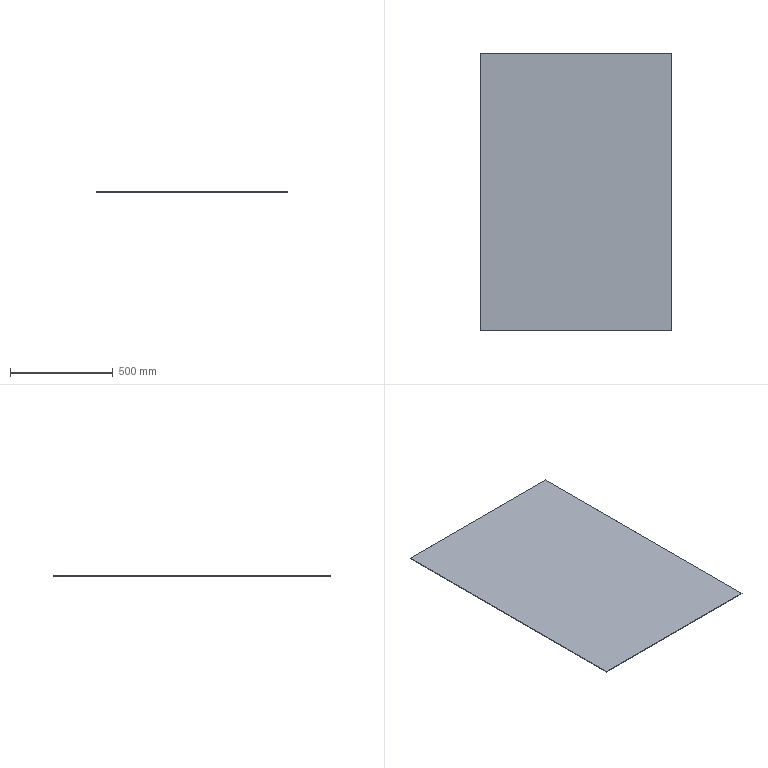Part | SolidWorks | features Extrusion 1 | 1 solid | 6 faces | box 935 x 1355 x 3 mm | volume 3800775 mm3 | plane 6
STEP:
#1=CARTESIAN_POINT('',(467.5,-677.5,0.));
#2=VERTEX_POINT('',#1);
#3=CARTESIAN_POINT('',(467.5,677.5,0.));
#4=VERTEX_POINT('',#3);
#5=CARTESIAN_POINT('',(467.5,677.5,0.));
#6=DIRECTION('',(0.,1.,0.));
#7=VECTOR('',#6,1000.);
#8=LINE('',#5,#7);
#9=EDGE_CURVE('',#2,#4,#8,.T.);
#10=ORIENTED_EDGE('',*,*,#9,.T.);
#11=CARTESIAN_POINT('',(467.5,677.5,3.));
#12=VERTEX_POINT('',#11);
#13=CARTESIAN_POINT('',(467.5,677.5,3.));
#14=DIRECTION('',(0.,0.,-1.));
#15=VECTOR('',#14,1000.);
#16=LINE('',#13,#15);
#17=EDGE_CURVE('',#12,#4,#16,.T.);
#18=ORIENTED_EDGE('',*,*,#17,.F.);
#19=CARTESIAN_POINT('',(467.5,-677.5,3.));
#20=VERTEX_POINT('',#19);
#21=CARTESIAN_POINT('',(467.5,677.5,3.));
#22=DIRECTION('',(0.,1.,0.));
#23=VECTOR('',#22,1000.);
#24=LINE('',#21,#23);
#25=EDGE_CURVE('',#20,#12,#24,.T.);
#26=ORIENTED_EDGE('',*,*,#25,.F.);
#27=CARTESIAN_POINT('',(467.5,-677.5,3.));
#28=DIRECTION('',(0.,0.,-1.));
#29=VECTOR('',#28,1000.);
#30=LINE('',#27,#29);
#31=EDGE_CURVE('',#20,#2,#30,.T.);
#32=ORIENTED_EDGE('',*,*,#31,.T.);
#33=EDGE_LOOP('',(#10,#18,#26,#32));
#34=FACE_OUTER_BOUND('',#33,.T.);
#35=CARTESIAN_POINT('',(467.5,677.5,3.));
#36=DIRECTION('',(-1.,0.,0.));
#37=DIRECTION('',(0.,-1.,0.));
#38=AXIS2_PLACEMENT_3D('',#35,#36,#37);
#39=PLANE('',#38);
#40=ADVANCED_FACE('',(#34),#39,.F.);
#41=CARTESIAN_POINT('',(-467.5,677.5,0.));
#42=VERTEX_POINT('',#41);
#43=CARTESIAN_POINT('',(-467.5,677.5,0.));
#44=DIRECTION('',(-1.,0.,0.));
#45=VECTOR('',#44,1000.);
#46=LINE('',#43,#45);
#47=EDGE_CURVE('',#4,#42,#46,.T.);
#48=ORIENTED_EDGE('',*,*,#47,.T.);
#49=CARTESIAN_POINT('',(-467.5,677.5,3.));
#50=VERTEX_POINT('',#49);
#51=CARTESIAN_POINT('',(-467.5,677.5,3.));
#52=DIRECTION('',(0.,0.,-1.));
#53=VECTOR('',#52,1000.);
#54=LINE('',#51,#53);
#55=EDGE_CURVE('',#50,#42,#54,.T.);
#56=ORIENTED_EDGE('',*,*,#55,.F.);
#57=CARTESIAN_POINT('',(-467.5,677.5,3.));
#58=DIRECTION('',(-1.,0.,0.));
#59=VECTOR('',#58,1000.);
#60=LINE('',#57,#59);
#61=EDGE_CURVE('',#12,#50,#60,.T.);
#62=ORIENTED_EDGE('',*,*,#61,.F.);
#63=ORIENTED_EDGE('',*,*,#17,.T.);
#64=EDGE_LOOP('',(#48,#56,#62,#63));
#65=FACE_OUTER_BOUND('',#64,.T.);
#66=CARTESIAN_POINT('',(-467.5,677.5,3.));
#67=DIRECTION('',(0.,-1.,0.));
#68=DIRECTION('',(0.,0.,-1.));
#69=AXIS2_PLACEMENT_3D('',#66,#67,#68);
#70=PLANE('',#69);
#71=ADVANCED_FACE('',(#65),#70,.F.);
#72=CARTESIAN_POINT('',(-467.5,-677.5,0.));
#73=VERTEX_POINT('',#72);
#74=CARTESIAN_POINT('',(-467.5,677.5,0.));
#75=DIRECTION('',(0.,-1.,0.));
#76=VECTOR('',#75,1000.);
#77=LINE('',#74,#76);
#78=EDGE_CURVE('',#42,#73,#77,.T.);
#79=ORIENTED_EDGE('',*,*,#78,.T.);
#80=CARTESIAN_POINT('',(-467.5,-677.5,3.));
#81=VERTEX_POINT('',#80);
#82=CARTESIAN_POINT('',(-467.5,-677.5,3.));
#83=DIRECTION('',(0.,0.,-1.));
#84=VECTOR('',#83,1000.);
#85=LINE('',#82,#84);
#86=EDGE_CURVE('',#81,#73,#85,.T.);
#87=ORIENTED_EDGE('',*,*,#86,.F.);
#88=CARTESIAN_POINT('',(-467.5,677.5,3.));
#89=DIRECTION('',(0.,-1.,0.));
#90=VECTOR('',#89,1000.);
#91=LINE('',#88,#90);
#92=EDGE_CURVE('',#50,#81,#91,.T.);
#93=ORIENTED_EDGE('',*,*,#92,.F.);
#94=ORIENTED_EDGE('',*,*,#55,.T.);
#95=EDGE_LOOP('',(#79,#87,#93,#94));
#96=FACE_OUTER_BOUND('',#95,.T.);
#97=CARTESIAN_POINT('',(-467.5,677.5,3.));
#98=DIRECTION('',(1.,0.,0.));
#99=DIRECTION('',(0.,0.,-1.));
#100=AXIS2_PLACEMENT_3D('',#97,#98,#99);
#101=PLANE('',#100);
#102=ADVANCED_FACE('',(#96),#101,.F.);
#103=CARTESIAN_POINT('',(-467.5,-677.5,0.));
#104=DIRECTION('',(1.,0.,0.));
#105=VECTOR('',#104,1000.);
#106=LINE('',#103,#105);
#107=EDGE_CURVE('',#73,#2,#106,.T.);
#108=ORIENTED_EDGE('',*,*,#107,.T.);
#109=ORIENTED_EDGE('',*,*,#31,.F.);
#110=CARTESIAN_POINT('',(-467.5,-677.5,3.));
#111=DIRECTION('',(1.,0.,0.));
#112=VECTOR('',#111,1000.);
#113=LINE('',#110,#112);
#114=EDGE_CURVE('',#81,#20,#113,.T.);
#115=ORIENTED_EDGE('',*,*,#114,.F.);
#116=ORIENTED_EDGE('',*,*,#86,.T.);
#117=EDGE_LOOP('',(#108,#109,#115,#116));
#118=FACE_OUTER_BOUND('',#117,.T.);
#119=CARTESIAN_POINT('',(-467.5,-677.5,3.));
#120=DIRECTION('',(0.,1.,0.));
#121=DIRECTION('',(0.,0.,1.));
#122=AXIS2_PLACEMENT_3D('',#119,#120,#121);
#123=PLANE('',#122);
#124=ADVANCED_FACE('',(#118),#123,.F.);
#125=ORIENTED_EDGE('',*,*,#25,.T.);
#126=ORIENTED_EDGE('',*,*,#61,.T.);
#127=ORIENTED_EDGE('',*,*,#92,.T.);
#128=ORIENTED_EDGE('',*,*,#114,.T.);
#129=EDGE_LOOP('',(#125,#126,#127,#128));
#130=FACE_OUTER_BOUND('',#129,.T.);
#131=CARTESIAN_POINT('',(0.,0.,3.));
#132=DIRECTION('',(0.,0.,1.));
#133=DIRECTION('',(1.,0.,0.));
#134=AXIS2_PLACEMENT_3D('',#131,#132,#133);
#135=PLANE('',#134);
#136=ADVANCED_FACE('',(#130),#135,.T.);
#137=ORIENTED_EDGE('',*,*,#9,.F.);
#138=ORIENTED_EDGE('',*,*,#107,.F.);
#139=ORIENTED_EDGE('',*,*,#78,.F.);
#140=ORIENTED_EDGE('',*,*,#47,.F.);
#141=EDGE_LOOP('',(#137,#138,#139,#140));
#142=FACE_OUTER_BOUND('',#141,.T.);
#143=CARTESIAN_POINT('',(0.,0.,0.));
#144=DIRECTION('',(0.,0.,1.));
#145=DIRECTION('',(1.,0.,0.));
#146=AXIS2_PLACEMENT_3D('',#143,#144,#145);
#147=PLANE('',#146);
#148=ADVANCED_FACE('',(#142),#147,.F.);
#149=CLOSED_SHELL('',(#40,#71,#102,#124,#136,#148));
#150=MANIFOLD_SOLID_BREP('',#149);
#151=CARTESIAN_POINT('',(0.,0.,0.));
#152=DIRECTION('',(0.,0.,1.));
#153=DIRECTION('',(1.,0.,0.));
#154=AXIS2_PLACEMENT_3D('',#151,#152,#153);
#155=(LENGTH_UNIT()NAMED_UNIT(*)SI_UNIT(.MILLI.,.METRE.));
#156=UNCERTAINTY_MEASURE_WITH_UNIT(LENGTH_MEASURE(0.00001),#155,'','');
#157=(NAMED_UNIT(*)PLANE_ANGLE_UNIT()SI_UNIT($,.RADIAN.));
#158=(NAMED_UNIT(*)SI_UNIT($,.STERADIAN.)SOLID_ANGLE_UNIT());
#159=(GEOMETRIC_REPRESENTATION_CONTEXT(3)GLOBAL_UNCERTAINTY_ASSIGNED_CONTEXT((#156))GLOBAL_UNIT_ASSIGNED_CONTEXT((#155,#157,#158))REPRESENTATION_CONTEXT('',''));
#160=ADVANCED_BREP_SHAPE_REPRESENTATION('',(#150,#154),#159);